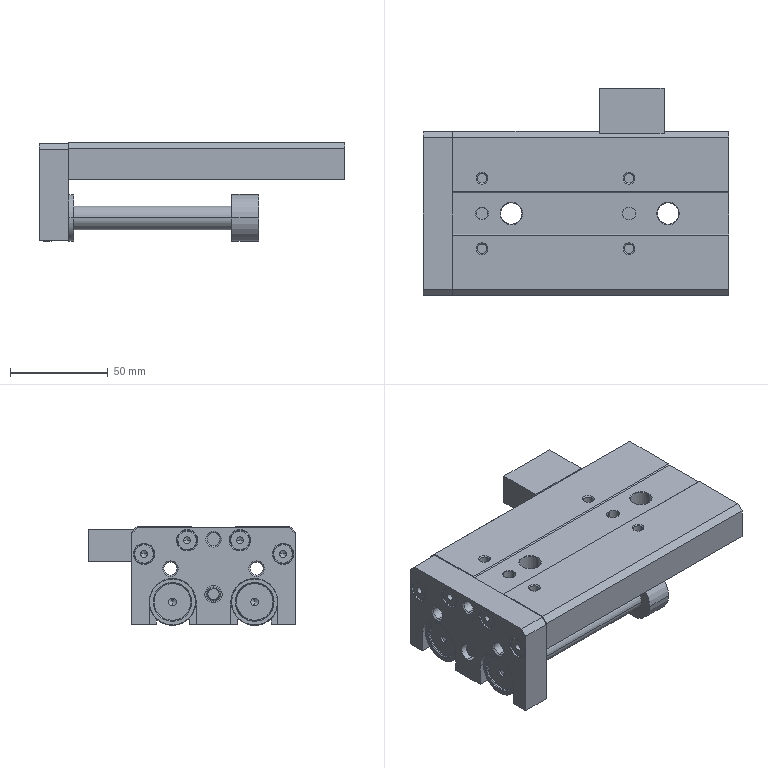Part | SolidWorks | features BaseBody 1 | 1 solid | 328 faces | box 156 x 106.01 x 50.5 mm | volume 274735 mm3 | plane 128 | cylinder 120 | cone 62 | spline 18 | commonest cylinder face diameters 10.5 x12 6.647 x10 23.8 x9 3.54 x8 4.917 x8 10 x8